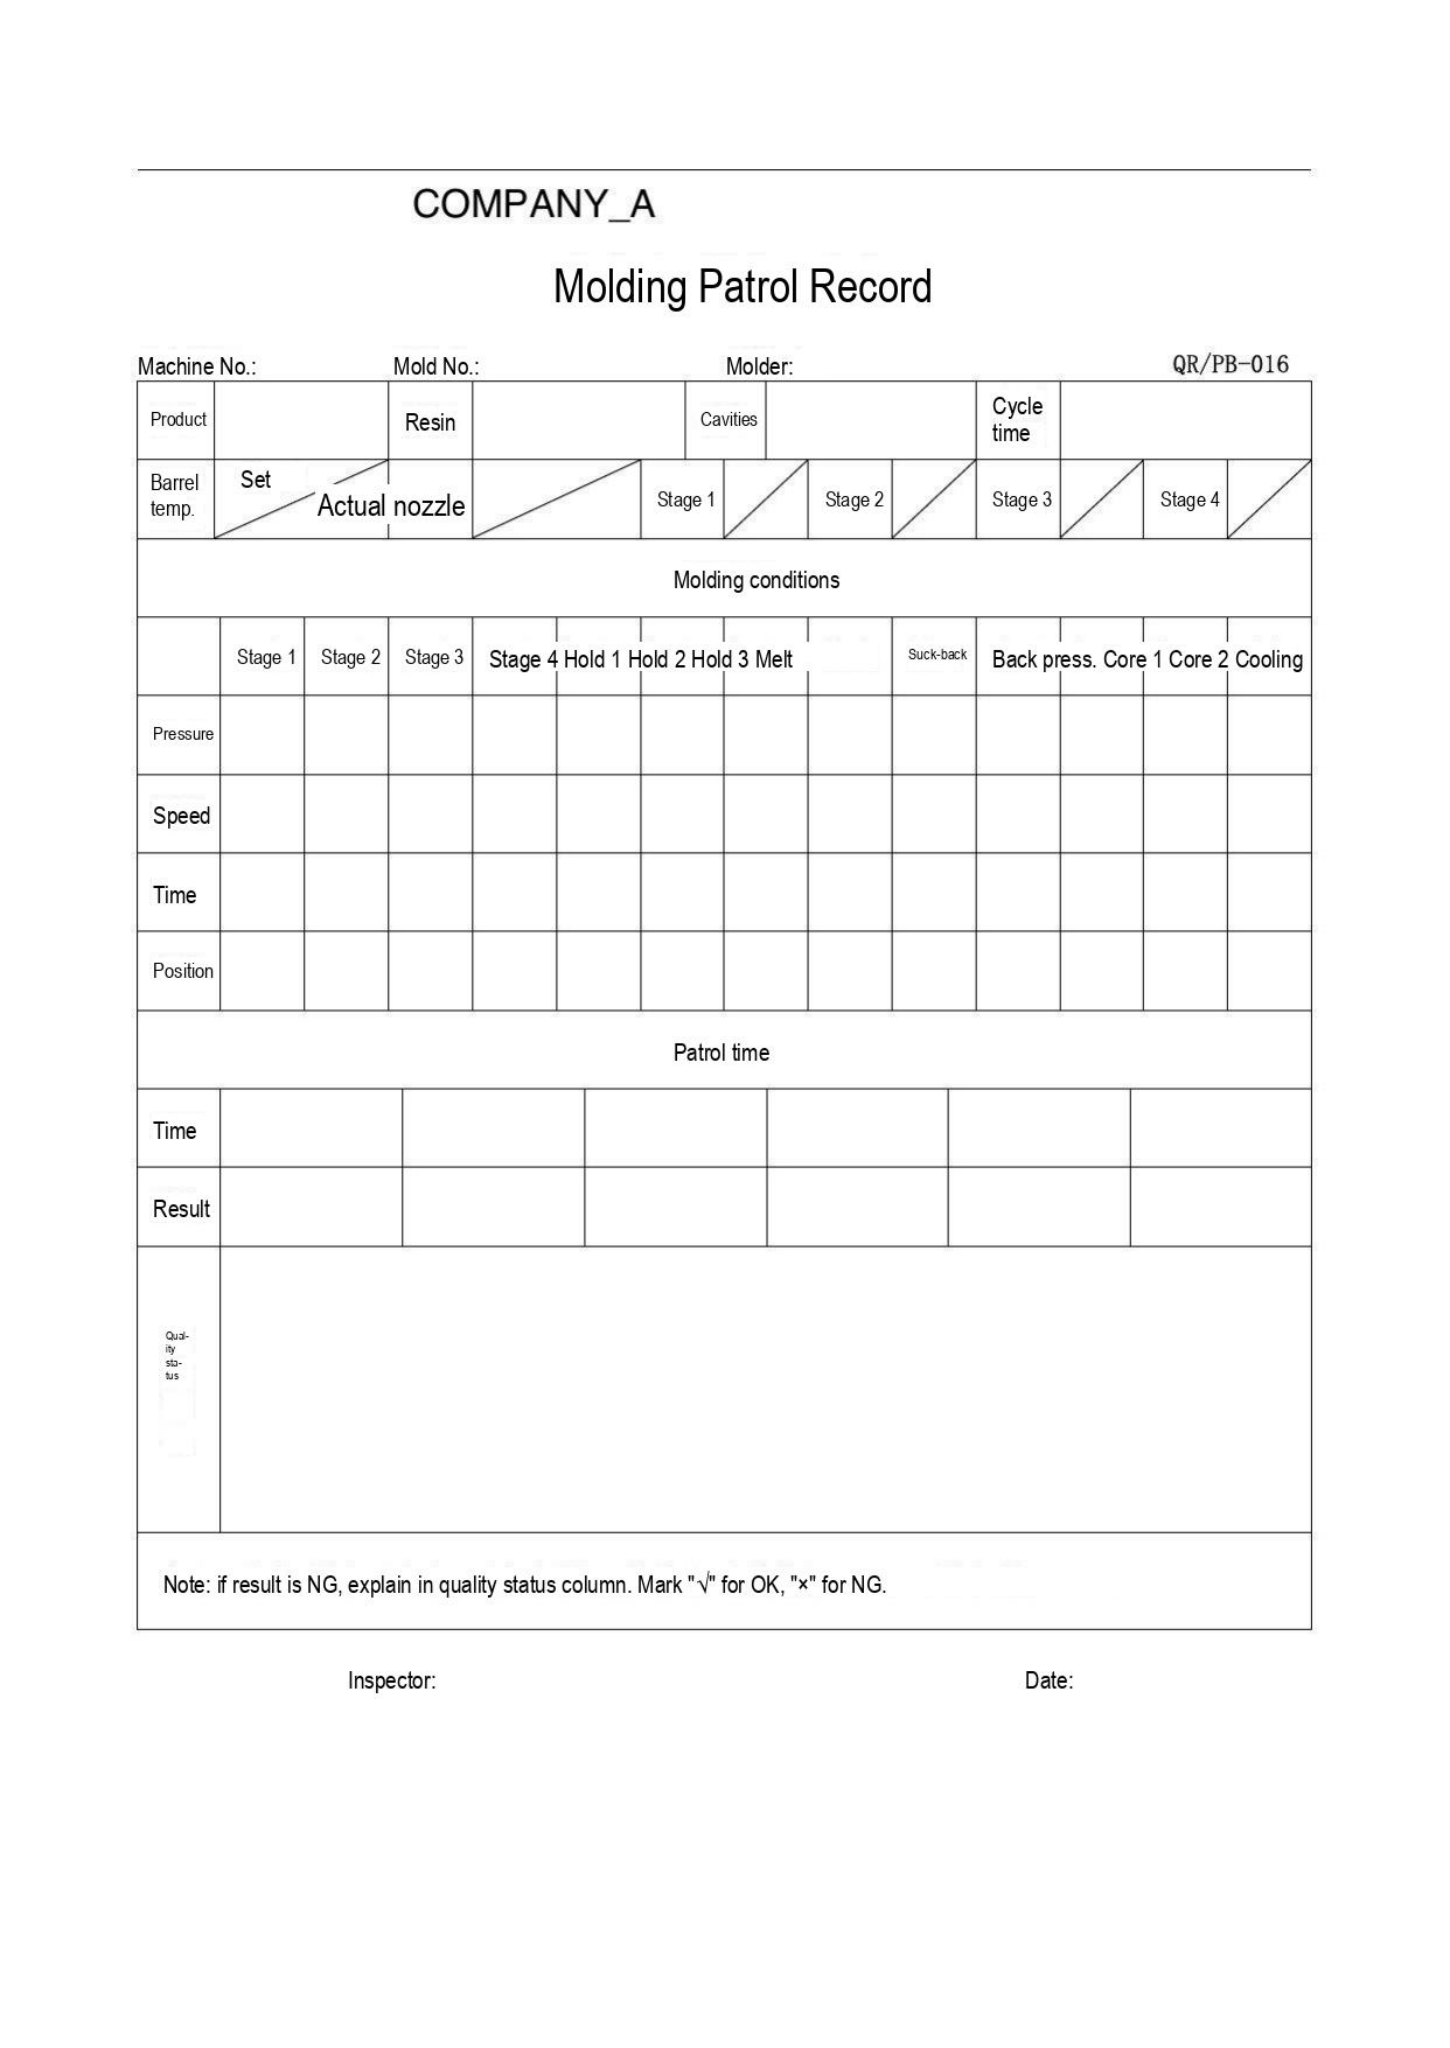COMPANY_A

Molding Patrol Record

Machine No.: Mold No.: Molder: QR/PB-016

| Product | | Resin | | Cavities | | Cycle time | |
|---|---|---|---|---|---|---|---|

| Barrel temp. | Set / Actual nozzle | | Stage 1 | | Stage 2 | | Stage 3 | | Stage 4 | |
|---|---|---|---|---|---|---|---|---|---|---|

Molding conditions

| | Stage 1 | Stage 2 | Stage 3 | Stage 4 | Hold 1 | Hold 2 | Hold 3 | Melt | Suck-back | Back press. | Core 1 | Core 2 | Cooling |
|---|---|---|---|---|---|---|---|---|---|---|---|---|---|
| Pressure | | | | | | | | | | | | | |
| Speed | | | | | | | | | | | | | |
| Time | | | | | | | | | | | | | |
| Position | | | | | | | | | | | | | |

Patrol time

| Time | | | | | | |
|---|---|---|---|---|---|---|
| Result | | | | | | |
| Quality status | | | | | | |

Note: if result is NG, explain in quality status column. Mark "√" for OK, "×" for NG.

Inspector: Date:
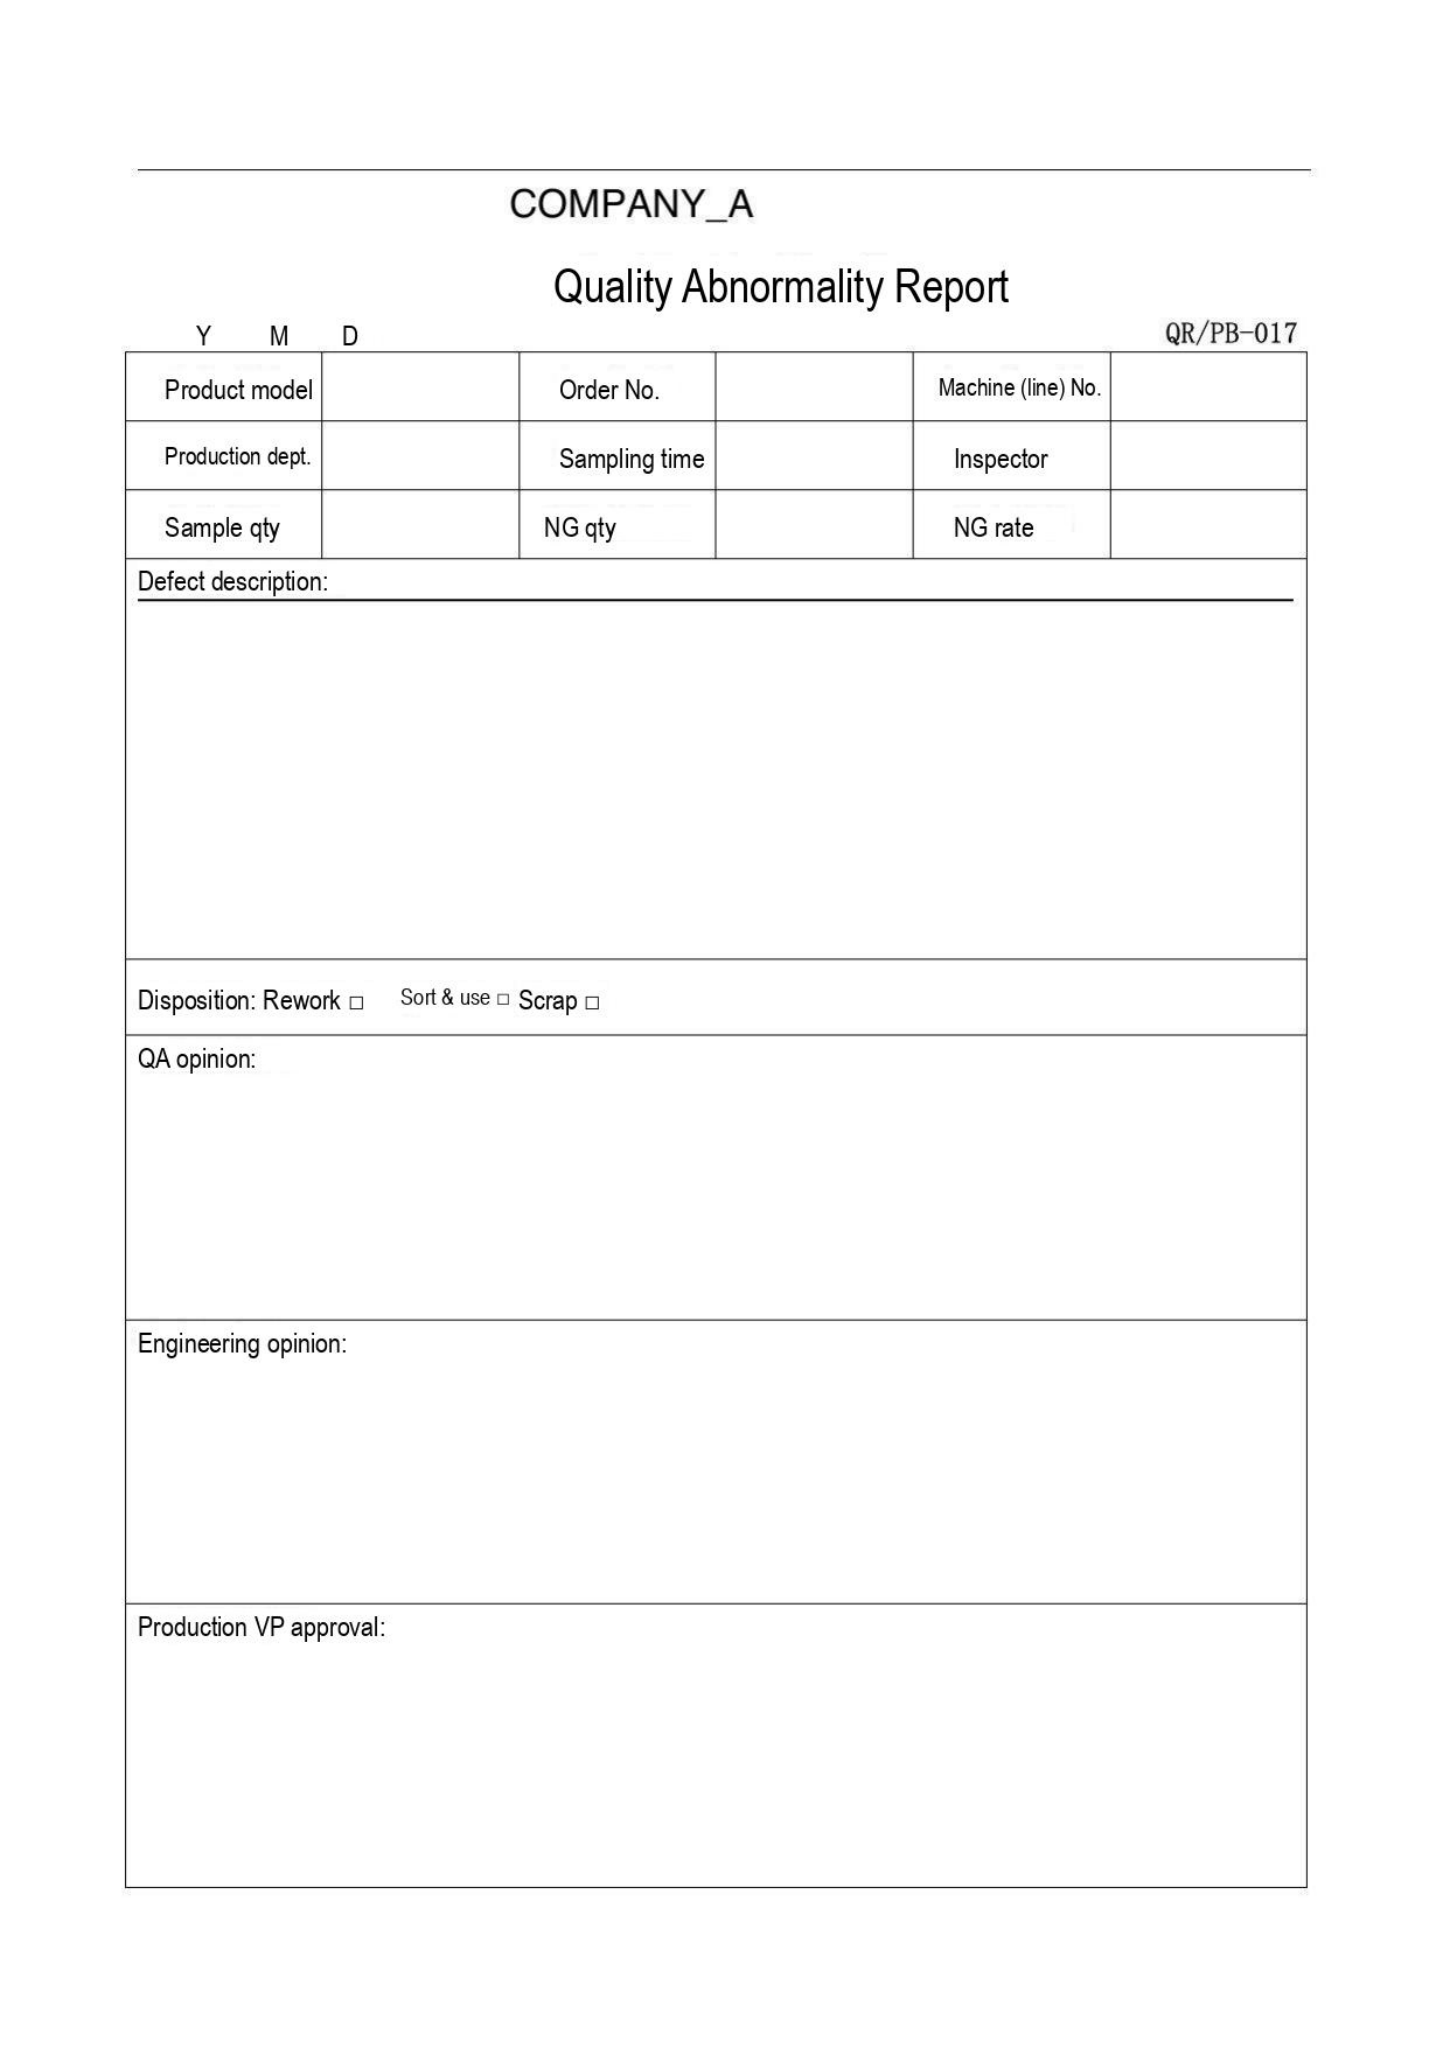COMPANY_A

Quality Abnormality Report

Y M D

QR/PB-017

| Product model | | Order No. | | Machine (line) No. | |
|---|---|---|---|---|---|
| Production dept. | | Sampling time | | Inspector | |
| Sample qty | | NG qty | | NG rate | |
| Defect description: | | | | | |
| Disposition: Rework □ Sort & use □ Scrap □ | | | | | |
| QA opinion: | | | | | |
| Engineering opinion: | | | | | |
| Production VP approval: | | | | | |
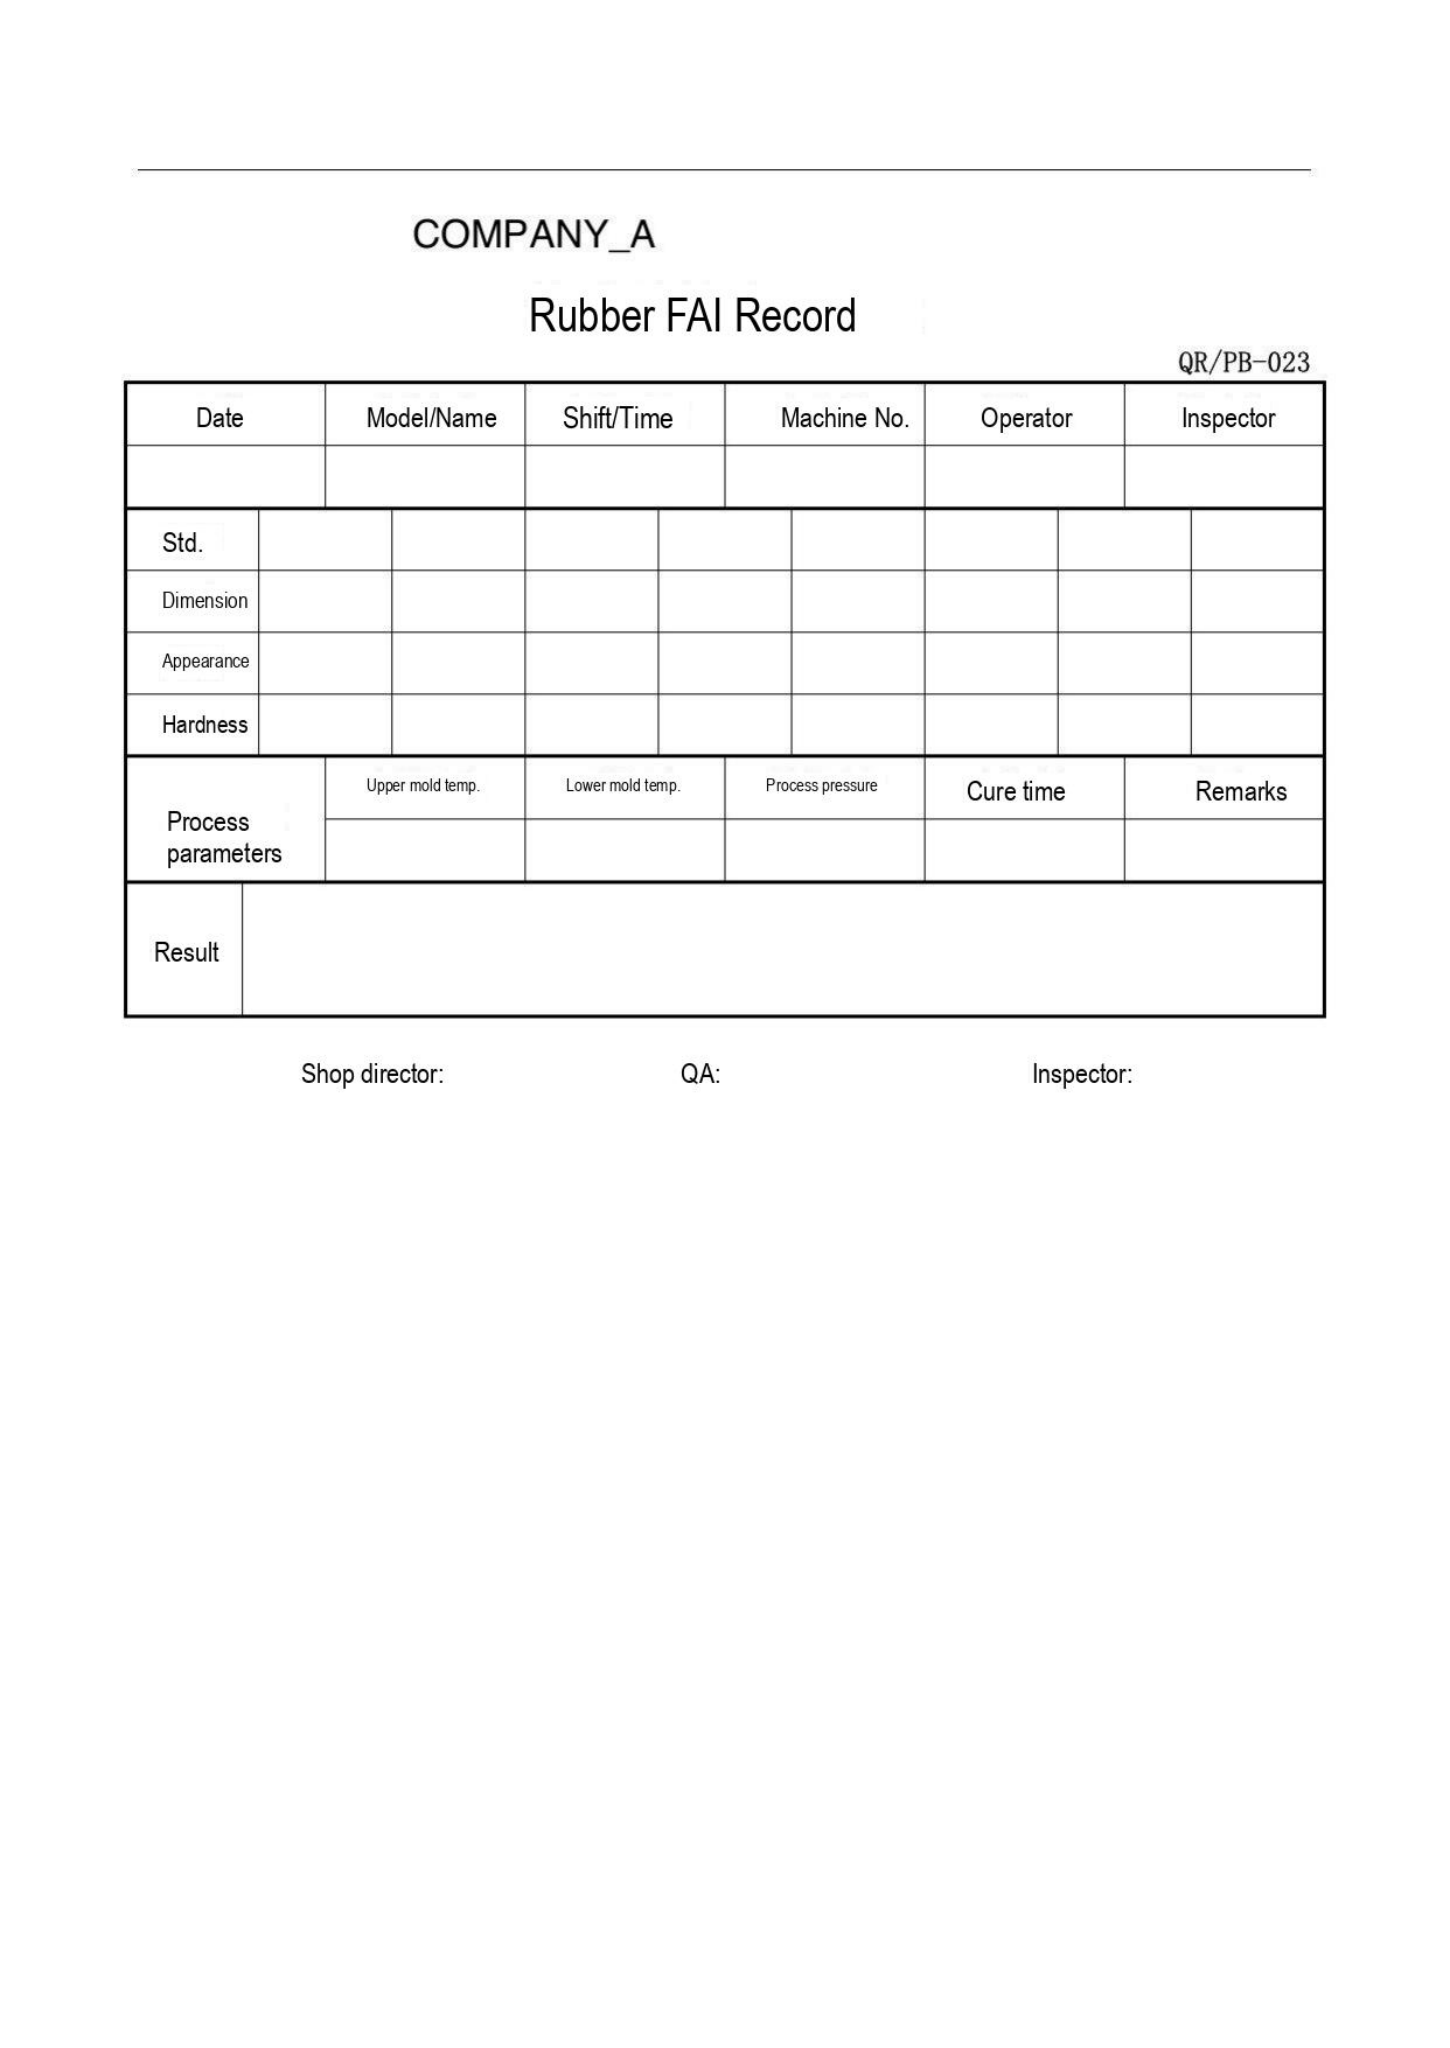COMPANY_A

Rubber FAI Record

QR/PB-023

| Date | Model/Name | Shift/Time | Machine No. | Operator | Inspector |
|---|---|---|---|---|---|
| | | | | | |

| Std. | | | | | | | | |
|---|---|---|---|---|---|---|---|---|
| Dimension | | | | | | | | |
| Appearance | | | | | | | | |
| Hardness | | | | | | | | |

| Process parameters | Upper mold temp. | Lower mold temp. | Process pressure | Cure time | Remarks |
|---|---|---|---|---|---|
| | | | | | |

| Result | |
|---|---|

Shop director: QA: Inspector:
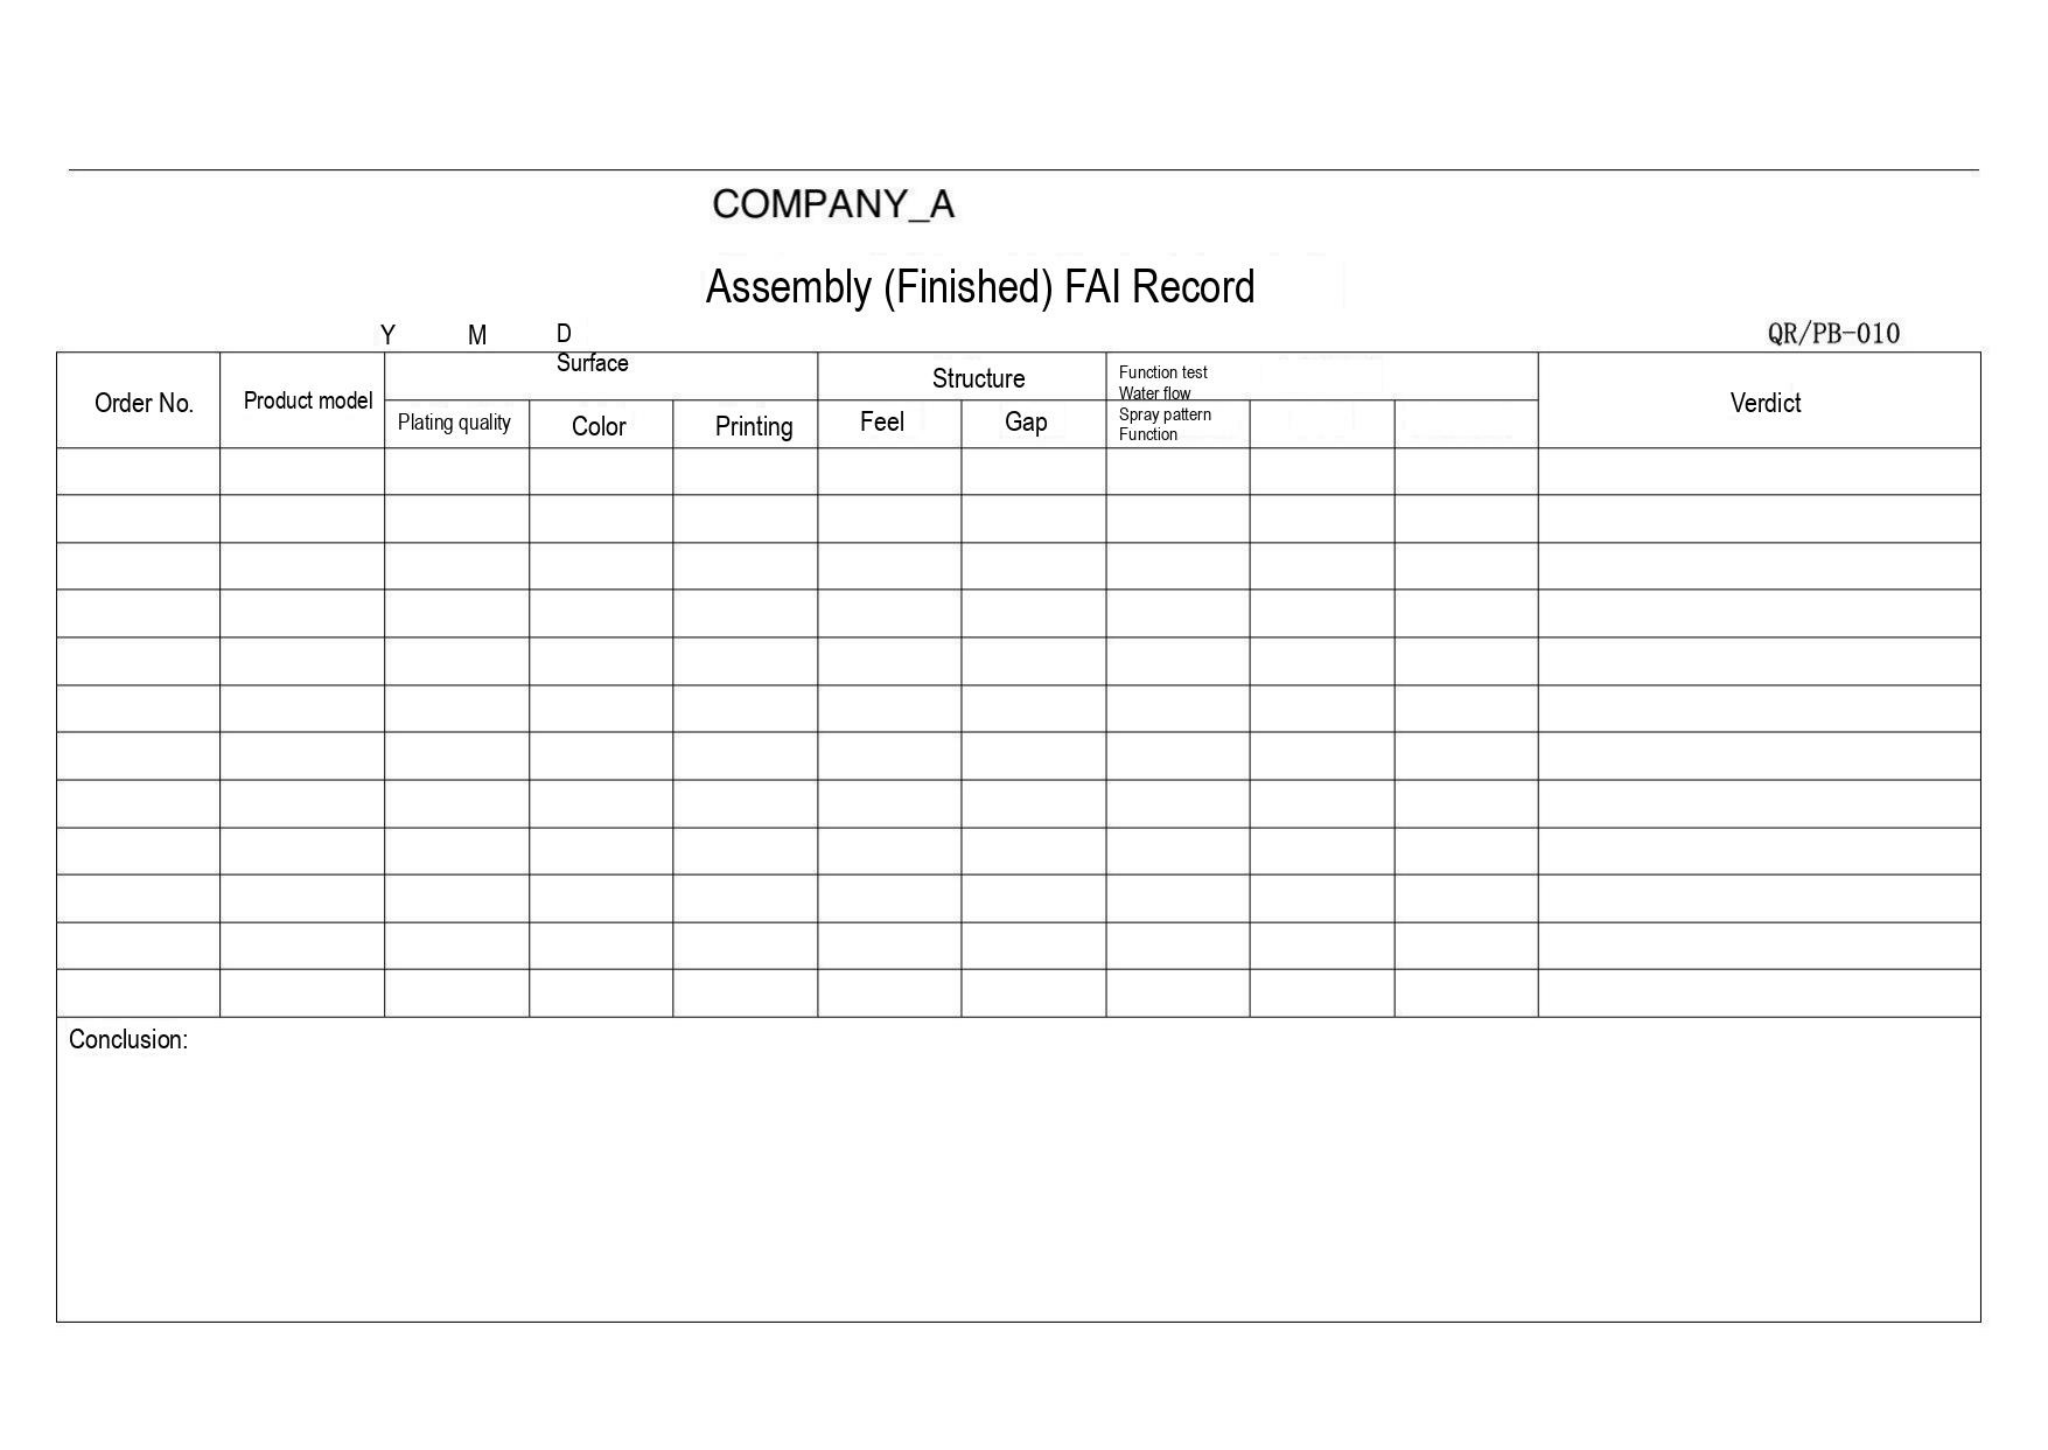COMPANY_A

Assembly (Finished) FAI Record

Y M D

QR/PB-010

| Order No. | Product model | Surface | | | Structure | | Function test | | | Verdict |
|---|---|---|---|---|---|---|---|---|---|---|
| | | Plating quality | Color | Printing | Feel | Gap | Water flow Spray pattern Function | | | |
| | | | | | | | | | | |
| | | | | | | | | | | |
| | | | | | | | | | | |
| | | | | | | | | | | |
| | | | | | | | | | | |
| | | | | | | | | | | |
| | | | | | | | | | | |
| | | | | | | | | | | |
| | | | | | | | | | | |
| | | | | | | | | | | |
| | | | | | | | | | | |
| | | | | | | | | | | |

Conclusion:
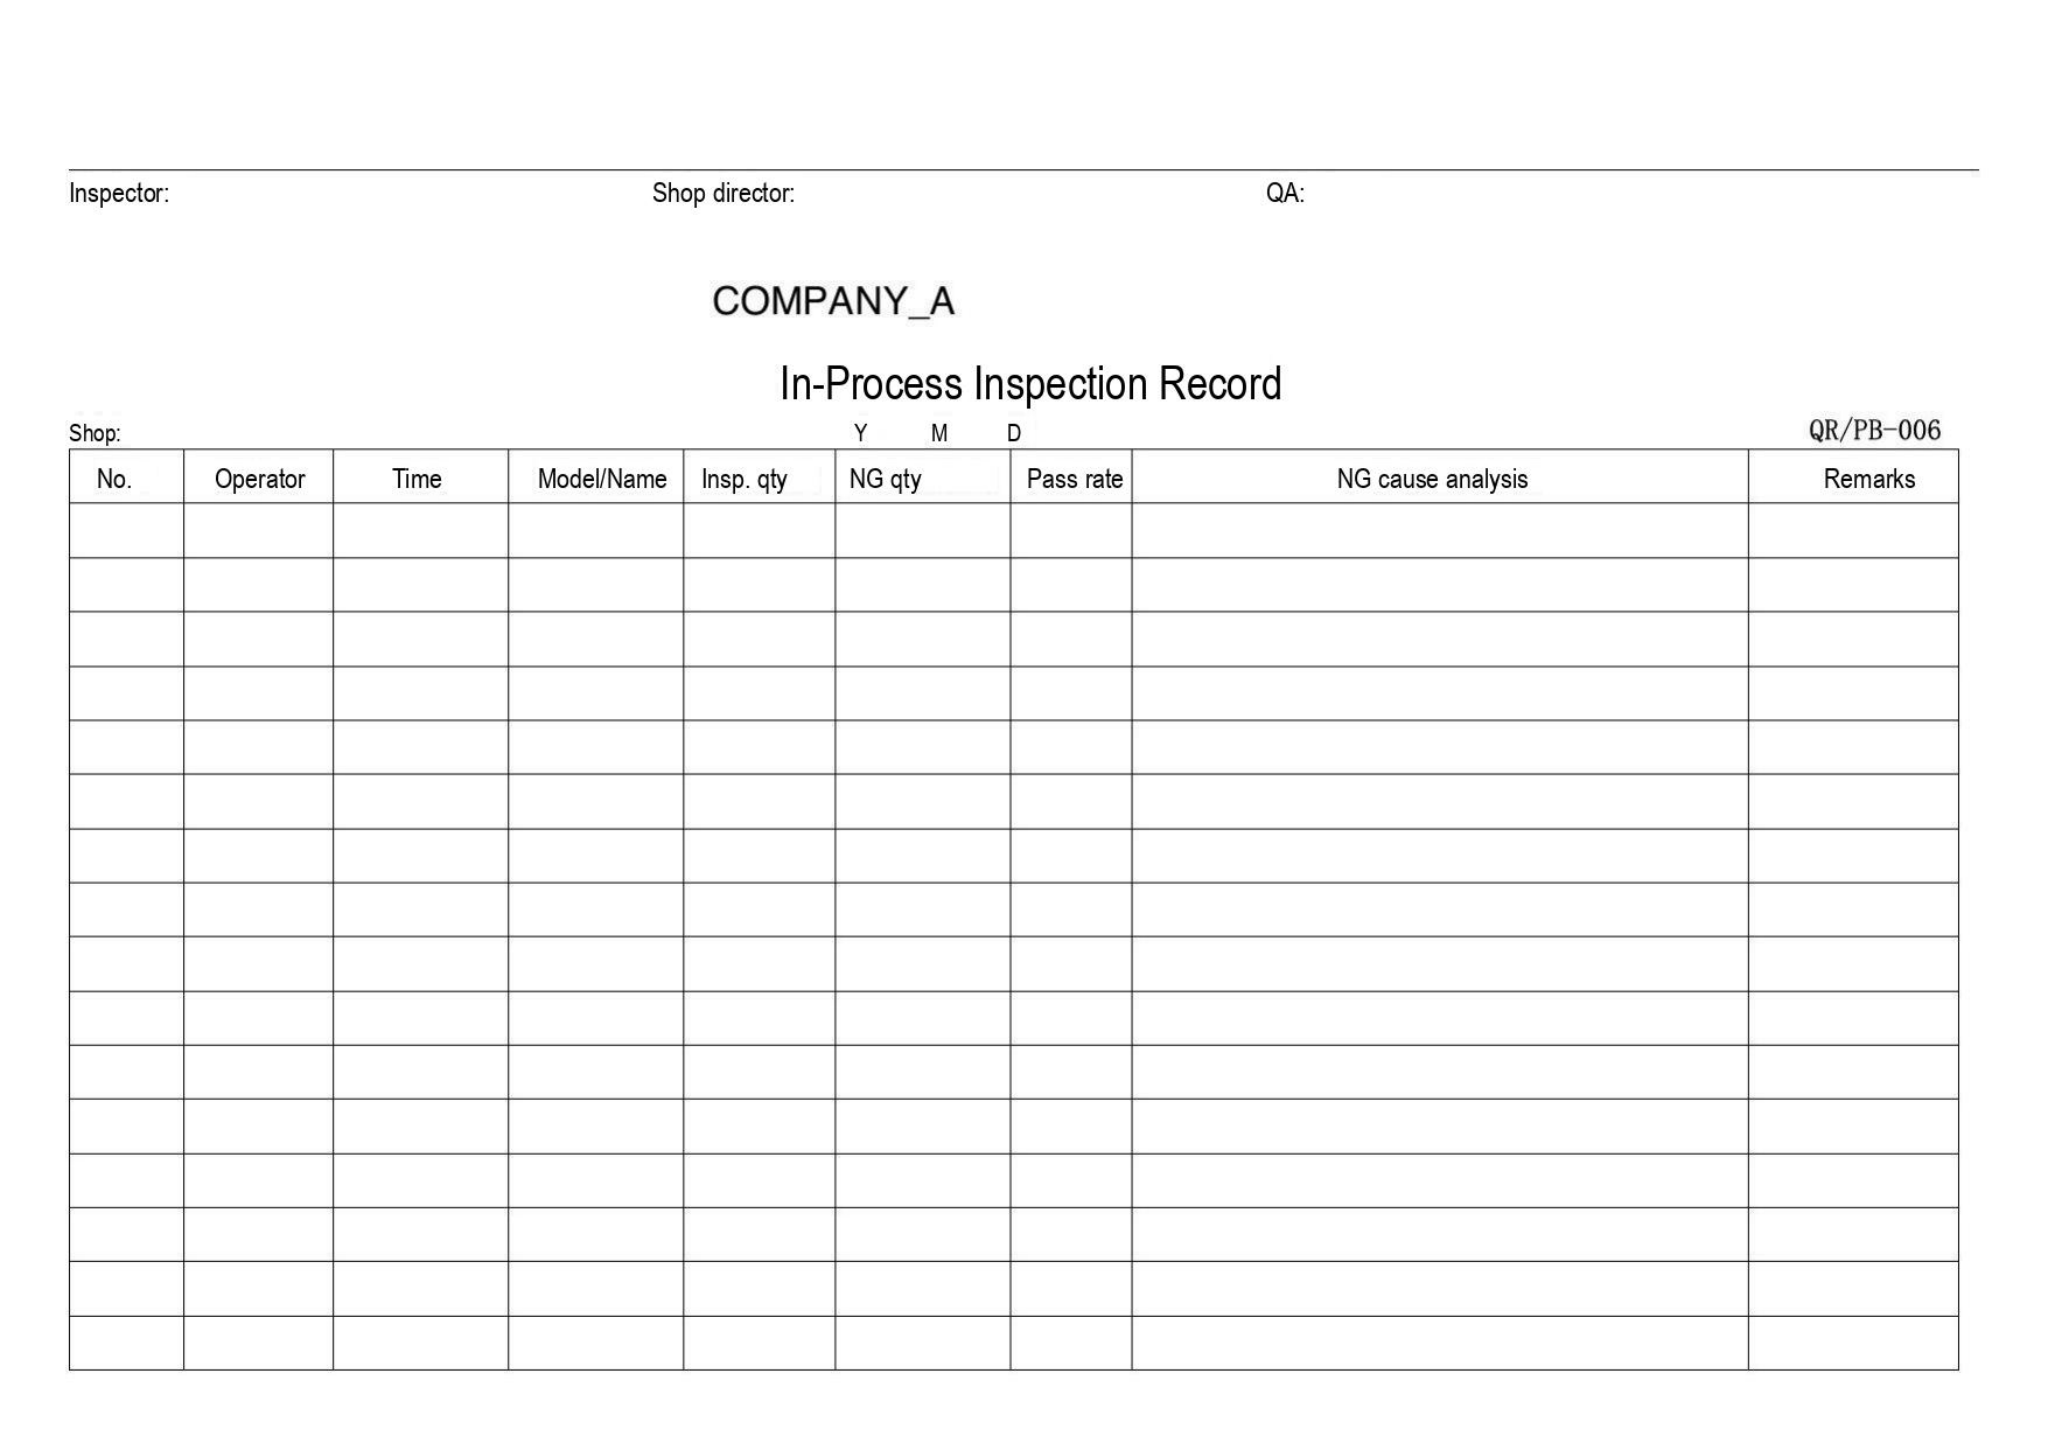Inspector: Shop director: QA:

COMPANY_A

In-Process Inspection Record

Shop: Y M D QR/PB-006

| No. | Operator | Time | Model/Name | Insp. qty | NG qty | Pass rate | NG cause analysis | Remarks |
|---|---|---|---|---|---|---|---|---|
| | | | | | | | | |
| | | | | | | | | |
| | | | | | | | | |
| | | | | | | | | |
| | | | | | | | | |
| | | | | | | | | |
| | | | | | | | | |
| | | | | | | | | |
| | | | | | | | | |
| | | | | | | | | |
| | | | | | | | | |
| | | | | | | | | |
| | | | | | | | | |
| | | | | | | | | |
| | | | | | | | | |
| | | | | | | | | |
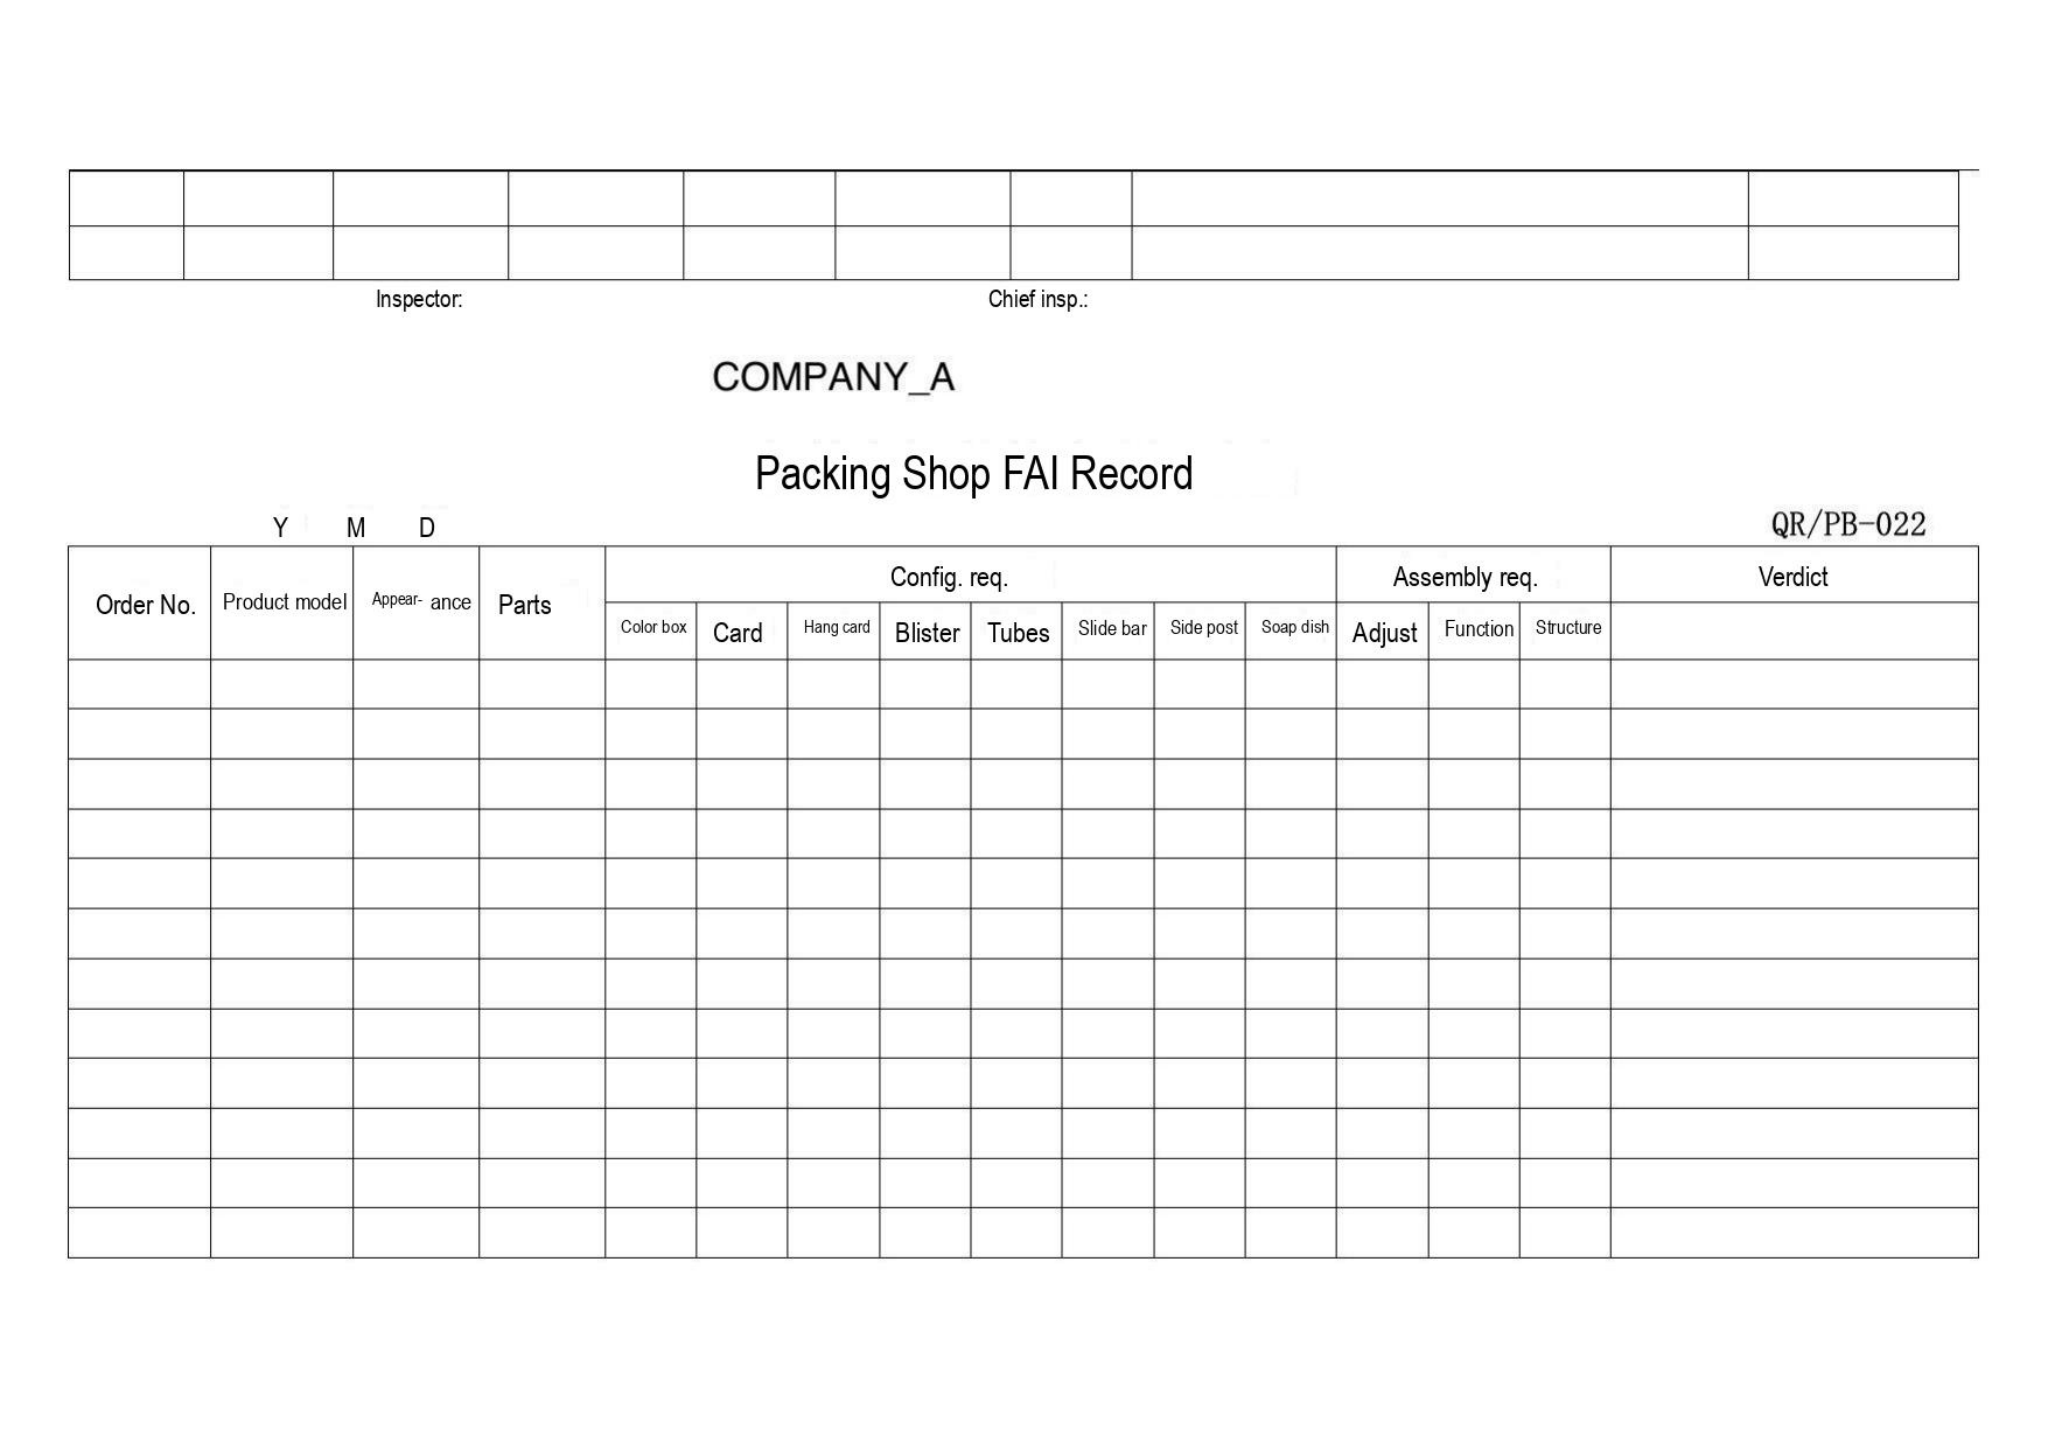|   |   |   |   |   |   |   |   |   |
|---|---|---|---|---|---|---|---|---|
|   |   |   |   |   |   |   |   |   |

Inspector: Chief insp.:

COMPANY_A

Packing Shop FAI Record

Y M D QR/PB-022

| Order No. | Product model | Appear- ance | Parts | Config. req. | | | | | | | | Assembly req. | | | Verdict |
|---|---|---|---|---|---|---|---|---|---|---|---|---|---|---|---|
| | | | | Color box | Card | Hang card | Blister | Tubes | Slide bar | Side post | Soap dish | Adjust | Function | Structure | |
| | | | | | | | | | | | | | | | |
| | | | | | | | | | | | | | | | |
| | | | | | | | | | | | | | | | |
| | | | | | | | | | | | | | | | |
| | | | | | | | | | | | | | | | |
| | | | | | | | | | | | | | | | |
| | | | | | | | | | | | | | | | |
| | | | | | | | | | | | | | | | |
| | | | | | | | | | | | | | | | |
| | | | | | | | | | | | | | | | |
| | | | | | | | | | | | | | | | |
| | | | | | | | | | | | | | | | |